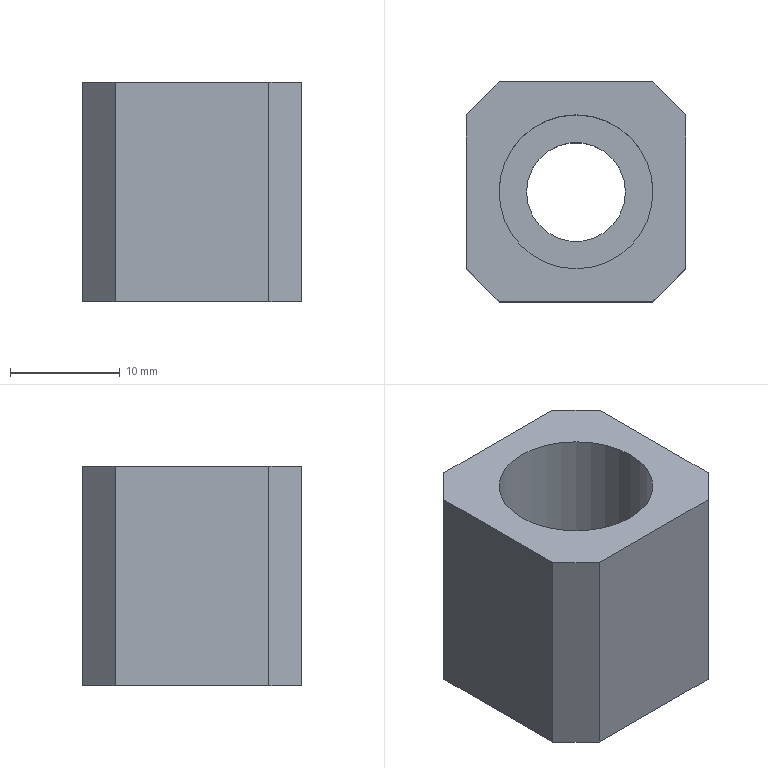Part | STEP file | 1_id270_x_t | 1 solid | 13 faces | box 20 x 20 x 20 mm | volume 5374 mm3 | plane 11 | cylinder 2 | commonest cylinder face diameters 9 x1 14 x1
STEP:
#1=CARTESIAN_POINT('',(0.,0.,0.));
#2=DIRECTION('',(0.,0.,1.));
#3=DIRECTION('',(1.,0.,0.));
#4=AXIS2_PLACEMENT_3D('',#1,#2,#3);
#5=CARTESIAN_POINT('',(740.075,184.5,-25.68));
#6=VERTEX_POINT('',#5);
#7=CARTESIAN_POINT('',(740.075,170.5,-25.68));
#8=VERTEX_POINT('',#7);
#9=CARTESIAN_POINT('',(740.075,188.5,-25.68));
#10=DIRECTION('',(0.,-1.,0.));
#11=VECTOR('',#10,1.);
#12=LINE('',#9,#11);
#13=CARTESIAN_POINT('',(740.075,188.5,-0.68));
#14=DIRECTION('',(1.,0.,0.));
#15=DIRECTION('',(0.,0.,-1.));
#16=AXIS2_PLACEMENT_3D('',#13,#14,#15);
#17=PLANE('',#16);
#18=CARTESIAN_POINT('',(25.,0.));
#19=DIRECTION('',(0.,-1.));
#20=VECTOR('',#19,1.);
#21=LINE('',#18,#20);
#22=(GEOMETRIC_REPRESENTATION_CONTEXT(2)PARAMETRIC_REPRESENTATION_CONTEXT()REPRESENTATION_CONTEXT('',''));
#23=DEFINITIONAL_REPRESENTATION('',(#21),#22);
#24=PCURVE('',#17,#23);
#25=CARTESIAN_POINT('',(740.075,166.5,-25.68));
#26=DIRECTION('',(0.,0.,1.));
#27=DIRECTION('',(1.,0.,0.));
#28=AXIS2_PLACEMENT_3D('',#25,#26,#27);
#29=PLANE('',#28);
#30=CARTESIAN_POINT('',(0.,22.));
#31=DIRECTION('',(0.,-1.));
#32=VECTOR('',#31,1.);
#33=LINE('',#30,#32);
#34=(GEOMETRIC_REPRESENTATION_CONTEXT(2)PARAMETRIC_REPRESENTATION_CONTEXT()REPRESENTATION_CONTEXT('',''));
#35=DEFINITIONAL_REPRESENTATION('',(#33),#34);
#36=PCURVE('',#29,#35);
#37=SURFACE_CURVE('',#12,(#24,#36),.PCURVE_S1.);
#38=EDGE_CURVE('',#6,#8,#37,.T.);
#39=ORIENTED_EDGE('',*,*,#38,.T.);
#40=CARTESIAN_POINT('',(740.075,170.5,-5.68));
#41=VERTEX_POINT('',#40);
#42=CARTESIAN_POINT('',(740.075,170.5,-0.68));
#43=DIRECTION('',(0.,0.,1.));
#44=VECTOR('',#43,1.);
#45=LINE('',#42,#44);
#46=CARTESIAN_POINT('',(0.,-18.));
#47=DIRECTION('',(-1.,0.));
#48=VECTOR('',#47,1.);
#49=LINE('',#46,#48);
#50=(GEOMETRIC_REPRESENTATION_CONTEXT(2)PARAMETRIC_REPRESENTATION_CONTEXT()REPRESENTATION_CONTEXT('',''));
#51=DEFINITIONAL_REPRESENTATION('',(#49),#50);
#52=PCURVE('',#17,#51);
#53=CARTESIAN_POINT('',(743.075,167.5,-0.68));
#54=DIRECTION('',(0.7071,0.7071,0.));
#55=DIRECTION('',(-0.7071,0.7071,0.));
#56=AXIS2_PLACEMENT_3D('',#53,#54,#55);
#57=PLANE('',#56);
#58=CARTESIAN_POINT('',(4.243,0.));
#59=DIRECTION('',(0.,1.));
#60=VECTOR('',#59,1.);
#61=LINE('',#58,#60);
#62=(GEOMETRIC_REPRESENTATION_CONTEXT(2)PARAMETRIC_REPRESENTATION_CONTEXT()REPRESENTATION_CONTEXT('',''));
#63=DEFINITIONAL_REPRESENTATION('',(#61),#62);
#64=PCURVE('',#57,#63);
#65=SURFACE_CURVE('',#45,(#52,#64),.PCURVE_S1.);
#66=EDGE_CURVE('',#8,#41,#65,.T.);
#67=ORIENTED_EDGE('',*,*,#66,.T.);
#68=CARTESIAN_POINT('',(740.075,184.5,-5.68));
#69=VERTEX_POINT('',#68);
#70=CARTESIAN_POINT('',(740.075,188.5,-5.68));
#71=DIRECTION('',(0.,-1.,0.));
#72=VECTOR('',#71,1.);
#73=LINE('',#70,#72);
#74=CARTESIAN_POINT('',(5.,0.));
#75=DIRECTION('',(0.,-1.));
#76=VECTOR('',#75,1.);
#77=LINE('',#74,#76);
#78=(GEOMETRIC_REPRESENTATION_CONTEXT(2)PARAMETRIC_REPRESENTATION_CONTEXT()REPRESENTATION_CONTEXT('',''));
#79=DEFINITIONAL_REPRESENTATION('',(#77),#78);
#80=PCURVE('',#17,#79);
#81=CARTESIAN_POINT('',(740.075,166.5,-5.68));
#82=DIRECTION('',(0.,0.,1.));
#83=DIRECTION('',(1.,0.,0.));
#84=AXIS2_PLACEMENT_3D('',#81,#82,#83);
#85=PLANE('',#84);
#86=CARTESIAN_POINT('',(0.,22.));
#87=DIRECTION('',(0.,-1.));
#88=VECTOR('',#87,1.);
#89=LINE('',#86,#88);
#90=(GEOMETRIC_REPRESENTATION_CONTEXT(2)PARAMETRIC_REPRESENTATION_CONTEXT()REPRESENTATION_CONTEXT('',''));
#91=DEFINITIONAL_REPRESENTATION('',(#89),#90);
#92=PCURVE('',#85,#91);
#93=SURFACE_CURVE('',#73,(#80,#92),.PCURVE_S1.);
#94=EDGE_CURVE('',#69,#41,#93,.T.);
#95=ORIENTED_EDGE('',*,*,#94,.F.);
#96=CARTESIAN_POINT('',(740.075,184.5,-0.68));
#97=DIRECTION('',(0.,0.,-1.));
#98=VECTOR('',#97,1.);
#99=LINE('',#96,#98);
#100=CARTESIAN_POINT('',(0.,-4.));
#101=DIRECTION('',(1.,0.));
#102=VECTOR('',#101,1.);
#103=LINE('',#100,#102);
#104=(GEOMETRIC_REPRESENTATION_CONTEXT(2)PARAMETRIC_REPRESENTATION_CONTEXT()REPRESENTATION_CONTEXT('',''));
#105=DEFINITIONAL_REPRESENTATION('',(#103),#104);
#106=PCURVE('',#17,#105);
#107=CARTESIAN_POINT('',(740.075,184.5,-0.68));
#108=DIRECTION('',(0.7071,-0.7071,0.));
#109=DIRECTION('',(0.7071,0.7071,0.));
#110=AXIS2_PLACEMENT_3D('',#107,#108,#109);
#111=PLANE('',#110);
#112=CARTESIAN_POINT('',(0.,0.));
#113=DIRECTION('',(0.,-1.));
#114=VECTOR('',#113,1.);
#115=LINE('',#112,#114);
#116=(GEOMETRIC_REPRESENTATION_CONTEXT(2)PARAMETRIC_REPRESENTATION_CONTEXT()REPRESENTATION_CONTEXT('',''));
#117=DEFINITIONAL_REPRESENTATION('',(#115),#116);
#118=PCURVE('',#111,#117);
#119=SURFACE_CURVE('',#99,(#106,#118),.PCURVE_S1.);
#120=EDGE_CURVE('',#69,#6,#119,.T.);
#121=ORIENTED_EDGE('',*,*,#120,.T.);
#122=EDGE_LOOP('',(#39,#67,#95,#121));
#123=FACE_BOUND('',#122,.T.);
#124=ADVANCED_FACE('',(#123),#17,.F.);
#125=CARTESIAN_POINT('',(743.075,167.5,-5.68));
#126=VERTEX_POINT('',#125);
#127=CARTESIAN_POINT('',(757.075,167.5,-5.68));
#128=VERTEX_POINT('',#127);
#129=CARTESIAN_POINT('',(740.075,167.5,-5.68));
#130=DIRECTION('',(1.,0.,0.));
#131=VECTOR('',#130,1.);
#132=LINE('',#129,#131);
#133=CARTESIAN_POINT('',(740.075,167.5,-0.68));
#134=DIRECTION('',(0.,1.,0.));
#135=DIRECTION('',(0.,0.,1.));
#136=AXIS2_PLACEMENT_3D('',#133,#134,#135);
#137=PLANE('',#136);
#138=CARTESIAN_POINT('',(-5.,0.));
#139=DIRECTION('',(0.,1.));
#140=VECTOR('',#139,1.);
#141=LINE('',#138,#140);
#142=(GEOMETRIC_REPRESENTATION_CONTEXT(2)PARAMETRIC_REPRESENTATION_CONTEXT()REPRESENTATION_CONTEXT('',''));
#143=DEFINITIONAL_REPRESENTATION('',(#141),#142);
#144=PCURVE('',#137,#143);
#145=CARTESIAN_POINT('',(0.,1.));
#146=DIRECTION('',(1.,0.));
#147=VECTOR('',#146,1.);
#148=LINE('',#145,#147);
#149=(GEOMETRIC_REPRESENTATION_CONTEXT(2)PARAMETRIC_REPRESENTATION_CONTEXT()REPRESENTATION_CONTEXT('',''));
#150=DEFINITIONAL_REPRESENTATION('',(#148),#149);
#151=PCURVE('',#85,#150);
#152=SURFACE_CURVE('',#132,(#144,#151),.PCURVE_S1.);
#153=EDGE_CURVE('',#126,#128,#152,.T.);
#154=ORIENTED_EDGE('',*,*,#153,.F.);
#155=CARTESIAN_POINT('',(743.075,167.5,-25.68));
#156=VERTEX_POINT('',#155);
#157=CARTESIAN_POINT('',(743.075,167.5,-0.68));
#158=DIRECTION('',(0.,0.,-1.));
#159=VECTOR('',#158,1.);
#160=LINE('',#157,#159);
#161=CARTESIAN_POINT('',(0.,3.));
#162=DIRECTION('',(-1.,0.));
#163=VECTOR('',#162,1.);
#164=LINE('',#161,#163);
#165=(GEOMETRIC_REPRESENTATION_CONTEXT(2)PARAMETRIC_REPRESENTATION_CONTEXT()REPRESENTATION_CONTEXT('',''));
#166=DEFINITIONAL_REPRESENTATION('',(#164),#165);
#167=PCURVE('',#137,#166);
#168=CARTESIAN_POINT('',(0.,0.));
#169=DIRECTION('',(0.,-1.));
#170=VECTOR('',#169,1.);
#171=LINE('',#168,#170);
#172=(GEOMETRIC_REPRESENTATION_CONTEXT(2)PARAMETRIC_REPRESENTATION_CONTEXT()REPRESENTATION_CONTEXT('',''));
#173=DEFINITIONAL_REPRESENTATION('',(#171),#172);
#174=PCURVE('',#57,#173);
#175=SURFACE_CURVE('',#160,(#167,#174),.PCURVE_S1.);
#176=EDGE_CURVE('',#126,#156,#175,.T.);
#177=ORIENTED_EDGE('',*,*,#176,.T.);
#178=CARTESIAN_POINT('',(757.075,167.5,-25.68));
#179=VERTEX_POINT('',#178);
#180=CARTESIAN_POINT('',(740.075,167.5,-25.68));
#181=DIRECTION('',(1.,0.,0.));
#182=VECTOR('',#181,1.);
#183=LINE('',#180,#182);
#184=CARTESIAN_POINT('',(-25.,0.));
#185=DIRECTION('',(0.,1.));
#186=VECTOR('',#185,1.);
#187=LINE('',#184,#186);
#188=(GEOMETRIC_REPRESENTATION_CONTEXT(2)PARAMETRIC_REPRESENTATION_CONTEXT()REPRESENTATION_CONTEXT('',''));
#189=DEFINITIONAL_REPRESENTATION('',(#187),#188);
#190=PCURVE('',#137,#189);
#191=CARTESIAN_POINT('',(0.,1.));
#192=DIRECTION('',(1.,0.));
#193=VECTOR('',#192,1.);
#194=LINE('',#191,#193);
#195=(GEOMETRIC_REPRESENTATION_CONTEXT(2)PARAMETRIC_REPRESENTATION_CONTEXT()REPRESENTATION_CONTEXT('',''));
#196=DEFINITIONAL_REPRESENTATION('',(#194),#195);
#197=PCURVE('',#29,#196);
#198=SURFACE_CURVE('',#183,(#190,#197),.PCURVE_S1.);
#199=EDGE_CURVE('',#156,#179,#198,.T.);
#200=ORIENTED_EDGE('',*,*,#199,.T.);
#201=CARTESIAN_POINT('',(757.075,167.5,-0.68));
#202=DIRECTION('',(0.,0.,1.));
#203=VECTOR('',#202,1.);
#204=LINE('',#201,#203);
#205=CARTESIAN_POINT('',(0.,17.));
#206=DIRECTION('',(1.,0.));
#207=VECTOR('',#206,1.);
#208=LINE('',#205,#207);
#209=(GEOMETRIC_REPRESENTATION_CONTEXT(2)PARAMETRIC_REPRESENTATION_CONTEXT()REPRESENTATION_CONTEXT('',''));
#210=DEFINITIONAL_REPRESENTATION('',(#208),#209);
#211=PCURVE('',#137,#210);
#212=CARTESIAN_POINT('',(760.075,170.5,-0.68));
#213=DIRECTION('',(-0.7071,0.7071,0.));
#214=DIRECTION('',(-0.7071,-0.7071,0.));
#215=AXIS2_PLACEMENT_3D('',#212,#213,#214);
#216=PLANE('',#215);
#217=CARTESIAN_POINT('',(4.243,0.));
#218=DIRECTION('',(0.,1.));
#219=VECTOR('',#218,1.);
#220=LINE('',#217,#219);
#221=(GEOMETRIC_REPRESENTATION_CONTEXT(2)PARAMETRIC_REPRESENTATION_CONTEXT()REPRESENTATION_CONTEXT('',''));
#222=DEFINITIONAL_REPRESENTATION('',(#220),#221);
#223=PCURVE('',#216,#222);
#224=SURFACE_CURVE('',#204,(#211,#223),.PCURVE_S1.);
#225=EDGE_CURVE('',#179,#128,#224,.T.);
#226=ORIENTED_EDGE('',*,*,#225,.T.);
#227=EDGE_LOOP('',(#154,#177,#200,#226));
#228=FACE_BOUND('',#227,.T.);
#229=ADVANCED_FACE('',(#228),#137,.F.);
#230=CARTESIAN_POINT('',(760.075,170.5,-5.68));
#231=VERTEX_POINT('',#230);
#232=CARTESIAN_POINT('',(760.075,184.5,-5.68));
#233=VERTEX_POINT('',#232);
#234=CARTESIAN_POINT('',(760.075,166.5,-5.68));
#235=DIRECTION('',(0.,1.,0.));
#236=VECTOR('',#235,1.);
#237=LINE('',#234,#236);
#238=CARTESIAN_POINT('',(760.075,166.5,-0.68));
#239=DIRECTION('',(-1.,0.,0.));
#240=DIRECTION('',(0.,0.,1.));
#241=AXIS2_PLACEMENT_3D('',#238,#239,#240);
#242=PLANE('',#241);
#243=CARTESIAN_POINT('',(-5.,0.));
#244=DIRECTION('',(0.,1.));
#245=VECTOR('',#244,1.);
#246=LINE('',#243,#245);
#247=(GEOMETRIC_REPRESENTATION_CONTEXT(2)PARAMETRIC_REPRESENTATION_CONTEXT()REPRESENTATION_CONTEXT('',''));
#248=DEFINITIONAL_REPRESENTATION('',(#246),#247);
#249=PCURVE('',#242,#248);
#250=CARTESIAN_POINT('',(20.,0.));
#251=DIRECTION('',(0.,1.));
#252=VECTOR('',#251,1.);
#253=LINE('',#250,#252);
#254=(GEOMETRIC_REPRESENTATION_CONTEXT(2)PARAMETRIC_REPRESENTATION_CONTEXT()REPRESENTATION_CONTEXT('',''));
#255=DEFINITIONAL_REPRESENTATION('',(#253),#254);
#256=PCURVE('',#85,#255);
#257=SURFACE_CURVE('',#237,(#249,#256),.PCURVE_S1.);
#258=EDGE_CURVE('',#231,#233,#257,.T.);
#259=ORIENTED_EDGE('',*,*,#258,.F.);
#260=CARTESIAN_POINT('',(760.075,170.5,-25.68));
#261=VERTEX_POINT('',#260);
#262=CARTESIAN_POINT('',(760.075,170.5,-0.68));
#263=DIRECTION('',(0.,0.,-1.));
#264=VECTOR('',#263,1.);
#265=LINE('',#262,#264);
#266=CARTESIAN_POINT('',(0.,4.));
#267=DIRECTION('',(-1.,0.));
#268=VECTOR('',#267,1.);
#269=LINE('',#266,#268);
#270=(GEOMETRIC_REPRESENTATION_CONTEXT(2)PARAMETRIC_REPRESENTATION_CONTEXT()REPRESENTATION_CONTEXT('',''));
#271=DEFINITIONAL_REPRESENTATION('',(#269),#270);
#272=PCURVE('',#242,#271);
#273=CARTESIAN_POINT('',(0.,0.));
#274=DIRECTION('',(0.,-1.));
#275=VECTOR('',#274,1.);
#276=LINE('',#273,#275);
#277=(GEOMETRIC_REPRESENTATION_CONTEXT(2)PARAMETRIC_REPRESENTATION_CONTEXT()REPRESENTATION_CONTEXT('',''));
#278=DEFINITIONAL_REPRESENTATION('',(#276),#277);
#279=PCURVE('',#216,#278);
#280=SURFACE_CURVE('',#265,(#272,#279),.PCURVE_S1.);
#281=EDGE_CURVE('',#231,#261,#280,.T.);
#282=ORIENTED_EDGE('',*,*,#281,.T.);
#283=CARTESIAN_POINT('',(760.075,184.5,-25.68));
#284=VERTEX_POINT('',#283);
#285=CARTESIAN_POINT('',(760.075,166.5,-25.68));
#286=DIRECTION('',(0.,1.,0.));
#287=VECTOR('',#286,1.);
#288=LINE('',#285,#287);
#289=CARTESIAN_POINT('',(-25.,0.));
#290=DIRECTION('',(0.,1.));
#291=VECTOR('',#290,1.);
#292=LINE('',#289,#291);
#293=(GEOMETRIC_REPRESENTATION_CONTEXT(2)PARAMETRIC_REPRESENTATION_CONTEXT()REPRESENTATION_CONTEXT('',''));
#294=DEFINITIONAL_REPRESENTATION('',(#292),#293);
#295=PCURVE('',#242,#294);
#296=CARTESIAN_POINT('',(20.,0.));
#297=DIRECTION('',(0.,1.));
#298=VECTOR('',#297,1.);
#299=LINE('',#296,#298);
#300=(GEOMETRIC_REPRESENTATION_CONTEXT(2)PARAMETRIC_REPRESENTATION_CONTEXT()REPRESENTATION_CONTEXT('',''));
#301=DEFINITIONAL_REPRESENTATION('',(#299),#300);
#302=PCURVE('',#29,#301);
#303=SURFACE_CURVE('',#288,(#295,#302),.PCURVE_S1.);
#304=EDGE_CURVE('',#261,#284,#303,.T.);
#305=ORIENTED_EDGE('',*,*,#304,.T.);
#306=CARTESIAN_POINT('',(760.075,184.5,-0.68));
#307=DIRECTION('',(0.,0.,1.));
#308=VECTOR('',#307,1.);
#309=LINE('',#306,#308);
#310=CARTESIAN_POINT('',(0.,18.));
#311=DIRECTION('',(1.,0.));
#312=VECTOR('',#311,1.);
#313=LINE('',#310,#312);
#314=(GEOMETRIC_REPRESENTATION_CONTEXT(2)PARAMETRIC_REPRESENTATION_CONTEXT()REPRESENTATION_CONTEXT('',''));
#315=DEFINITIONAL_REPRESENTATION('',(#313),#314);
#316=PCURVE('',#242,#315);
#317=CARTESIAN_POINT('',(757.075,187.5,-0.68));
#318=DIRECTION('',(-0.7071,-0.7071,0.));
#319=DIRECTION('',(0.7071,-0.7071,0.));
#320=AXIS2_PLACEMENT_3D('',#317,#318,#319);
#321=PLANE('',#320);
#322=CARTESIAN_POINT('',(4.243,0.));
#323=DIRECTION('',(0.,1.));
#324=VECTOR('',#323,1.);
#325=LINE('',#322,#324);
#326=(GEOMETRIC_REPRESENTATION_CONTEXT(2)PARAMETRIC_REPRESENTATION_CONTEXT()REPRESENTATION_CONTEXT('',''));
#327=DEFINITIONAL_REPRESENTATION('',(#325),#326);
#328=PCURVE('',#321,#327);
#329=SURFACE_CURVE('',#309,(#316,#328),.PCURVE_S1.);
#330=EDGE_CURVE('',#284,#233,#329,.T.);
#331=ORIENTED_EDGE('',*,*,#330,.T.);
#332=EDGE_LOOP('',(#259,#282,#305,#331));
#333=FACE_BOUND('',#332,.T.);
#334=ADVANCED_FACE('',(#333),#242,.F.);
#335=CARTESIAN_POINT('',(757.075,187.5,-25.68));
#336=VERTEX_POINT('',#335);
#337=CARTESIAN_POINT('',(743.075,187.5,-25.68));
#338=VERTEX_POINT('',#337);
#339=CARTESIAN_POINT('',(760.075,187.5,-25.68));
#340=DIRECTION('',(-1.,0.,0.));
#341=VECTOR('',#340,1.);
#342=LINE('',#339,#341);
#343=CARTESIAN_POINT('',(760.075,187.5,-0.68));
#344=DIRECTION('',(0.,-1.,0.));
#345=DIRECTION('',(0.,0.,-1.));
#346=AXIS2_PLACEMENT_3D('',#343,#344,#345);
#347=PLANE('',#346);
#348=CARTESIAN_POINT('',(25.,0.));
#349=DIRECTION('',(0.,-1.));
#350=VECTOR('',#349,1.);
#351=LINE('',#348,#350);
#352=(GEOMETRIC_REPRESENTATION_CONTEXT(2)PARAMETRIC_REPRESENTATION_CONTEXT()REPRESENTATION_CONTEXT('',''));
#353=DEFINITIONAL_REPRESENTATION('',(#351),#352);
#354=PCURVE('',#347,#353);
#355=CARTESIAN_POINT('',(20.,21.));
#356=DIRECTION('',(-1.,0.));
#357=VECTOR('',#356,1.);
#358=LINE('',#355,#357);
#359=(GEOMETRIC_REPRESENTATION_CONTEXT(2)PARAMETRIC_REPRESENTATION_CONTEXT()REPRESENTATION_CONTEXT('',''));
#360=DEFINITIONAL_REPRESENTATION('',(#358),#359);
#361=PCURVE('',#29,#360);
#362=SURFACE_CURVE('',#342,(#354,#361),.PCURVE_S1.);
#363=EDGE_CURVE('',#336,#338,#362,.T.);
#364=ORIENTED_EDGE('',*,*,#363,.T.);
#365=CARTESIAN_POINT('',(743.075,187.5,-5.68));
#366=VERTEX_POINT('',#365);
#367=CARTESIAN_POINT('',(743.075,187.5,-0.68));
#368=DIRECTION('',(0.,0.,1.));
#369=VECTOR('',#368,1.);
#370=LINE('',#367,#369);
#371=CARTESIAN_POINT('',(0.,-17.));
#372=DIRECTION('',(-1.,0.));
#373=VECTOR('',#372,1.);
#374=LINE('',#371,#373);
#375=(GEOMETRIC_REPRESENTATION_CONTEXT(2)PARAMETRIC_REPRESENTATION_CONTEXT()REPRESENTATION_CONTEXT('',''));
#376=DEFINITIONAL_REPRESENTATION('',(#374),#375);
#377=PCURVE('',#347,#376);
#378=CARTESIAN_POINT('',(4.243,0.));
#379=DIRECTION('',(0.,1.));
#380=VECTOR('',#379,1.);
#381=LINE('',#378,#380);
#382=(GEOMETRIC_REPRESENTATION_CONTEXT(2)PARAMETRIC_REPRESENTATION_CONTEXT()REPRESENTATION_CONTEXT('',''));
#383=DEFINITIONAL_REPRESENTATION('',(#381),#382);
#384=PCURVE('',#111,#383);
#385=SURFACE_CURVE('',#370,(#377,#384),.PCURVE_S1.);
#386=EDGE_CURVE('',#338,#366,#385,.T.);
#387=ORIENTED_EDGE('',*,*,#386,.T.);
#388=CARTESIAN_POINT('',(757.075,187.5,-5.68));
#389=VERTEX_POINT('',#388);
#390=CARTESIAN_POINT('',(760.075,187.5,-5.68));
#391=DIRECTION('',(-1.,0.,0.));
#392=VECTOR('',#391,1.);
#393=LINE('',#390,#392);
#394=CARTESIAN_POINT('',(5.,0.));
#395=DIRECTION('',(0.,-1.));
#396=VECTOR('',#395,1.);
#397=LINE('',#394,#396);
#398=(GEOMETRIC_REPRESENTATION_CONTEXT(2)PARAMETRIC_REPRESENTATION_CONTEXT()REPRESENTATION_CONTEXT('',''));
#399=DEFINITIONAL_REPRESENTATION('',(#397),#398);
#400=PCURVE('',#347,#399);
#401=CARTESIAN_POINT('',(20.,21.));
#402=DIRECTION('',(-1.,0.));
#403=VECTOR('',#402,1.);
#404=LINE('',#401,#403);
#405=(GEOMETRIC_REPRESENTATION_CONTEXT(2)PARAMETRIC_REPRESENTATION_CONTEXT()REPRESENTATION_CONTEXT('',''));
#406=DEFINITIONAL_REPRESENTATION('',(#404),#405);
#407=PCURVE('',#85,#406);
#408=SURFACE_CURVE('',#393,(#400,#407),.PCURVE_S1.);
#409=EDGE_CURVE('',#389,#366,#408,.T.);
#410=ORIENTED_EDGE('',*,*,#409,.F.);
#411=CARTESIAN_POINT('',(757.075,187.5,-0.68));
#412=DIRECTION('',(0.,0.,-1.));
#413=VECTOR('',#412,1.);
#414=LINE('',#411,#413);
#415=CARTESIAN_POINT('',(0.,-3.));
#416=DIRECTION('',(1.,0.));
#417=VECTOR('',#416,1.);
#418=LINE('',#415,#417);
#419=(GEOMETRIC_REPRESENTATION_CONTEXT(2)PARAMETRIC_REPRESENTATION_CONTEXT()REPRESENTATION_CONTEXT('',''));
#420=DEFINITIONAL_REPRESENTATION('',(#418),#419);
#421=PCURVE('',#347,#420);
#422=CARTESIAN_POINT('',(0.,0.));
#423=DIRECTION('',(0.,-1.));
#424=VECTOR('',#423,1.);
#425=LINE('',#422,#424);
#426=(GEOMETRIC_REPRESENTATION_CONTEXT(2)PARAMETRIC_REPRESENTATION_CONTEXT()REPRESENTATION_CONTEXT('',''));
#427=DEFINITIONAL_REPRESENTATION('',(#425),#426);
#428=PCURVE('',#321,#427);
#429=SURFACE_CURVE('',#414,(#421,#428),.PCURVE_S1.);
#430=EDGE_CURVE('',#389,#336,#429,.T.);
#431=ORIENTED_EDGE('',*,*,#430,.T.);
#432=EDGE_LOOP('',(#364,#387,#410,#431));
#433=FACE_BOUND('',#432,.T.);
#434=ADVANCED_FACE('',(#433),#347,.F.);
#435=CARTESIAN_POINT('',(743.075,177.5,-5.68));
#436=VERTEX_POINT('',#435);
#437=CARTESIAN_POINT('',(750.075,177.5,-5.68));
#438=DIRECTION('',(0.,0.,-1.));
#439=DIRECTION('',(-1.,0.,0.));
#440=AXIS2_PLACEMENT_3D('',#437,#438,#439);
#441=CIRCLE('',#440,7.);
#442=CARTESIAN_POINT('',(3.,11.));
#443=CARTESIAN_POINT('',(3.,23.124));
#444=CARTESIAN_POINT('',(13.5,17.062));
#445=CARTESIAN_POINT('',(24.,11.));
#446=CARTESIAN_POINT('',(13.5,4.938));
#447=CARTESIAN_POINT('',(3.,-1.124));
#448=CARTESIAN_POINT('',(3.,11.));
#449=(BOUNDED_CURVE()B_SPLINE_CURVE(2,(#442,#443,#444,#445,#446,#447,#448),.UNSPECIFIED.,.T.,.F.)B_SPLINE_CURVE_WITH_KNOTS((1,2,2,2,2,1),(-2.094,0.,2.094,4.189,6.283,8.378),.UNSPECIFIED.)CURVE()GEOMETRIC_REPRESENTATION_ITEM()RATIONAL_B_SPLINE_CURVE((1.,0.5,1.,0.5,1.,0.5,1.))REPRESENTATION_ITEM(''));
#450=(GEOMETRIC_REPRESENTATION_CONTEXT(2)PARAMETRIC_REPRESENTATION_CONTEXT()REPRESENTATION_CONTEXT('',''));
#451=DEFINITIONAL_REPRESENTATION('',(#449),#450);
#452=PCURVE('',#85,#451);
#453=CARTESIAN_POINT('',(750.075,177.5,-5.68));
#454=DIRECTION('',(0.,0.,-1.));
#455=DIRECTION('',(-1.,0.,0.));
#456=AXIS2_PLACEMENT_3D('',#453,#454,#455);
#457=CYLINDRICAL_SURFACE('',#456,7.);
#458=CARTESIAN_POINT('',(0.,0.));
#459=DIRECTION('',(1.,0.));
#460=VECTOR('',#459,1.);
#461=LINE('',#458,#460);
#462=(GEOMETRIC_REPRESENTATION_CONTEXT(2)PARAMETRIC_REPRESENTATION_CONTEXT()REPRESENTATION_CONTEXT('',''));
#463=DEFINITIONAL_REPRESENTATION('',(#461),#462);
#464=PCURVE('',#457,#463);
#465=SURFACE_CURVE('',#441,(#452,#464),.PCURVE_S1.);
#466=EDGE_CURVE('',#436,#436,#465,.T.);
#467=ORIENTED_EDGE('',*,*,#466,.T.);
#468=EDGE_LOOP('',(#467));
#469=FACE_BOUND('',#468,.T.);
#470=ORIENTED_EDGE('',*,*,#94,.T.);
#471=CARTESIAN_POINT('',(742.075,168.5,-5.68));
#472=DIRECTION('',(0.7071,-0.7071,0.));
#473=VECTOR('',#472,1.);
#474=LINE('',#471,#473);
#475=CARTESIAN_POINT('',(2.,2.));
#476=DIRECTION('',(0.7071,-0.7071));
#477=VECTOR('',#476,1.);
#478=LINE('',#475,#477);
#479=(GEOMETRIC_REPRESENTATION_CONTEXT(2)PARAMETRIC_REPRESENTATION_CONTEXT()REPRESENTATION_CONTEXT('',''));
#480=DEFINITIONAL_REPRESENTATION('',(#478),#479);
#481=PCURVE('',#85,#480);
#482=CARTESIAN_POINT('',(1.414,-5.));
#483=DIRECTION('',(-1.,0.));
#484=VECTOR('',#483,1.);
#485=LINE('',#482,#484);
#486=(GEOMETRIC_REPRESENTATION_CONTEXT(2)PARAMETRIC_REPRESENTATION_CONTEXT()REPRESENTATION_CONTEXT('',''));
#487=DEFINITIONAL_REPRESENTATION('',(#485),#486);
#488=PCURVE('',#57,#487);
#489=SURFACE_CURVE('',#474,(#481,#488),.PCURVE_S1.);
#490=EDGE_CURVE('',#41,#126,#489,.T.);
#491=ORIENTED_EDGE('',*,*,#490,.T.);
#492=ORIENTED_EDGE('',*,*,#153,.T.);
#493=CARTESIAN_POINT('',(748.075,158.5,-5.68));
#494=DIRECTION('',(0.7071,0.7071,0.));
#495=VECTOR('',#494,1.);
#496=LINE('',#493,#495);
#497=CARTESIAN_POINT('',(8.,-8.));
#498=DIRECTION('',(0.7071,0.7071));
#499=VECTOR('',#498,1.);
#500=LINE('',#497,#499);
#501=(GEOMETRIC_REPRESENTATION_CONTEXT(2)PARAMETRIC_REPRESENTATION_CONTEXT()REPRESENTATION_CONTEXT('',''));
#502=DEFINITIONAL_REPRESENTATION('',(#500),#501);
#503=PCURVE('',#85,#502);
#504=CARTESIAN_POINT('',(16.971,-5.));
#505=DIRECTION('',(-1.,0.));
#506=VECTOR('',#505,1.);
#507=LINE('',#504,#506);
#508=(GEOMETRIC_REPRESENTATION_CONTEXT(2)PARAMETRIC_REPRESENTATION_CONTEXT()REPRESENTATION_CONTEXT('',''));
#509=DEFINITIONAL_REPRESENTATION('',(#507),#508);
#510=PCURVE('',#216,#509);
#511=SURFACE_CURVE('',#496,(#503,#510),.PCURVE_S1.);
#512=EDGE_CURVE('',#128,#231,#511,.T.);
#513=ORIENTED_EDGE('',*,*,#512,.T.);
#514=ORIENTED_EDGE('',*,*,#258,.T.);
#515=CARTESIAN_POINT('',(759.075,185.5,-5.68));
#516=DIRECTION('',(-0.7071,0.7071,0.));
#517=VECTOR('',#516,1.);
#518=LINE('',#515,#517);
#519=CARTESIAN_POINT('',(19.,19.));
#520=DIRECTION('',(-0.7071,0.7071));
#521=VECTOR('',#520,1.);
#522=LINE('',#519,#521);
#523=(GEOMETRIC_REPRESENTATION_CONTEXT(2)PARAMETRIC_REPRESENTATION_CONTEXT()REPRESENTATION_CONTEXT('',''));
#524=DEFINITIONAL_REPRESENTATION('',(#522),#523);
#525=PCURVE('',#85,#524);
#526=CARTESIAN_POINT('',(2.828,-5.));
#527=DIRECTION('',(-1.,0.));
#528=VECTOR('',#527,1.);
#529=LINE('',#526,#528);
#530=(GEOMETRIC_REPRESENTATION_CONTEXT(2)PARAMETRIC_REPRESENTATION_CONTEXT()REPRESENTATION_CONTEXT('',''));
#531=DEFINITIONAL_REPRESENTATION('',(#529),#530);
#532=PCURVE('',#321,#531);
#533=SURFACE_CURVE('',#518,(#525,#532),.PCURVE_S1.);
#534=EDGE_CURVE('',#233,#389,#533,.T.);
#535=ORIENTED_EDGE('',*,*,#534,.T.);
#536=ORIENTED_EDGE('',*,*,#409,.T.);
#537=CARTESIAN_POINT('',(731.075,175.5,-5.68));
#538=DIRECTION('',(-0.7071,-0.7071,0.));
#539=VECTOR('',#538,1.);
#540=LINE('',#537,#539);
#541=CARTESIAN_POINT('',(-9.,9.));
#542=DIRECTION('',(-0.7071,-0.7071));
#543=VECTOR('',#542,1.);
#544=LINE('',#541,#543);
#545=(GEOMETRIC_REPRESENTATION_CONTEXT(2)PARAMETRIC_REPRESENTATION_CONTEXT()REPRESENTATION_CONTEXT('',''));
#546=DEFINITIONAL_REPRESENTATION('',(#544),#545);
#547=PCURVE('',#85,#546);
#548=CARTESIAN_POINT('',(-12.728,-5.));
#549=DIRECTION('',(-1.,0.));
#550=VECTOR('',#549,1.);
#551=LINE('',#548,#550);
#552=(GEOMETRIC_REPRESENTATION_CONTEXT(2)PARAMETRIC_REPRESENTATION_CONTEXT()REPRESENTATION_CONTEXT('',''));
#553=DEFINITIONAL_REPRESENTATION('',(#551),#552);
#554=PCURVE('',#111,#553);
#555=SURFACE_CURVE('',#540,(#547,#554),.PCURVE_S1.);
#556=EDGE_CURVE('',#366,#69,#555,.T.);
#557=ORIENTED_EDGE('',*,*,#556,.T.);
#558=EDGE_LOOP('',(#470,#491,#492,#513,#514,#535,#536,#557));
#559=FACE_BOUND('',#558,.T.);
#560=ADVANCED_FACE('',(#469,#559),#85,.T.);
#561=CARTESIAN_POINT('',(754.575,177.5,-25.68));
#562=VERTEX_POINT('',#561);
#563=CARTESIAN_POINT('',(745.575,177.5,-25.68));
#564=VERTEX_POINT('',#563);
#565=CARTESIAN_POINT('',(750.075,177.5,-25.68));
#566=DIRECTION('',(0.,0.,1.));
#567=DIRECTION('',(1.,0.,0.));
#568=AXIS2_PLACEMENT_3D('',#565,#566,#567);
#569=CIRCLE('',#568,4.5);
#570=CARTESIAN_POINT('',(10.,11.));
#571=DIRECTION('',(1.,0.));
#572=AXIS2_PLACEMENT_2D('',#570,#571);
#573=CIRCLE('',#572,4.5);
#574=(GEOMETRIC_REPRESENTATION_CONTEXT(2)PARAMETRIC_REPRESENTATION_CONTEXT()REPRESENTATION_CONTEXT('',''));
#575=DEFINITIONAL_REPRESENTATION('',(#573),#574);
#576=PCURVE('',#29,#575);
#577=CARTESIAN_POINT('',(750.075,177.5,-105.68));
#578=DIRECTION('',(0.,0.,-1.));
#579=DIRECTION('',(-1.,0.,0.));
#580=AXIS2_PLACEMENT_3D('',#577,#578,#579);
#581=CYLINDRICAL_SURFACE('',#580,4.5);
#582=CARTESIAN_POINT('',(3.142,-80.));
#583=DIRECTION('',(-1.,0.));
#584=VECTOR('',#583,1.);
#585=LINE('',#582,#584);
#586=(GEOMETRIC_REPRESENTATION_CONTEXT(2)PARAMETRIC_REPRESENTATION_CONTEXT()REPRESENTATION_CONTEXT('',''));
#587=DEFINITIONAL_REPRESENTATION('',(#585),#586);
#588=PCURVE('',#581,#587);
#589=SURFACE_CURVE('',#569,(#576,#588),.PCURVE_S1.);
#590=EDGE_CURVE('',#562,#564,#589,.T.);
#591=ORIENTED_EDGE('',*,*,#590,.T.);
#592=CARTESIAN_POINT('',(750.075,177.5,-25.68));
#593=DIRECTION('',(0.,0.,1.));
#594=DIRECTION('',(1.,0.,0.));
#595=AXIS2_PLACEMENT_3D('',#592,#593,#594);
#596=CIRCLE('',#595,4.5);
#597=CARTESIAN_POINT('',(10.,11.));
#598=DIRECTION('',(1.,0.));
#599=AXIS2_PLACEMENT_2D('',#597,#598);
#600=CIRCLE('',#599,4.5);
#601=(GEOMETRIC_REPRESENTATION_CONTEXT(2)PARAMETRIC_REPRESENTATION_CONTEXT()REPRESENTATION_CONTEXT('',''));
#602=DEFINITIONAL_REPRESENTATION('',(#600),#601);
#603=PCURVE('',#29,#602);
#604=CARTESIAN_POINT('',(9.425,-80.));
#605=DIRECTION('',(-1.,0.));
#606=VECTOR('',#605,1.);
#607=LINE('',#604,#606);
#608=(GEOMETRIC_REPRESENTATION_CONTEXT(2)PARAMETRIC_REPRESENTATION_CONTEXT()REPRESENTATION_CONTEXT('',''));
#609=DEFINITIONAL_REPRESENTATION('',(#607),#608);
#610=PCURVE('',#581,#609);
#611=SURFACE_CURVE('',#596,(#603,#610),.PCURVE_S1.);
#612=EDGE_CURVE('',#564,#562,#611,.T.);
#613=ORIENTED_EDGE('',*,*,#612,.T.);
#614=EDGE_LOOP('',(#591,#613));
#615=FACE_BOUND('',#614,.T.);
#616=ORIENTED_EDGE('',*,*,#199,.F.);
#617=CARTESIAN_POINT('',(743.075,167.5,-25.68));
#618=DIRECTION('',(-0.7071,0.7071,0.));
#619=VECTOR('',#618,1.);
#620=LINE('',#617,#619);
#621=CARTESIAN_POINT('',(3.,1.));
#622=DIRECTION('',(-0.7071,0.7071));
#623=VECTOR('',#622,1.);
#624=LINE('',#621,#623);
#625=(GEOMETRIC_REPRESENTATION_CONTEXT(2)PARAMETRIC_REPRESENTATION_CONTEXT()REPRESENTATION_CONTEXT('',''));
#626=DEFINITIONAL_REPRESENTATION('',(#624),#625);
#627=PCURVE('',#29,#626);
#628=CARTESIAN_POINT('',(0.,-25.));
#629=DIRECTION('',(1.,0.));
#630=VECTOR('',#629,1.);
#631=LINE('',#628,#630);
#632=(GEOMETRIC_REPRESENTATION_CONTEXT(2)PARAMETRIC_REPRESENTATION_CONTEXT()REPRESENTATION_CONTEXT('',''));
#633=DEFINITIONAL_REPRESENTATION('',(#631),#632);
#634=PCURVE('',#57,#633);
#635=SURFACE_CURVE('',#620,(#627,#634),.PCURVE_S1.);
#636=EDGE_CURVE('',#156,#8,#635,.T.);
#637=ORIENTED_EDGE('',*,*,#636,.T.);
#638=ORIENTED_EDGE('',*,*,#38,.F.);
#639=CARTESIAN_POINT('',(740.075,184.5,-25.68));
#640=DIRECTION('',(0.7071,0.7071,0.));
#641=VECTOR('',#640,1.);
#642=LINE('',#639,#641);
#643=CARTESIAN_POINT('',(0.,18.));
#644=DIRECTION('',(0.7071,0.7071));
#645=VECTOR('',#644,1.);
#646=LINE('',#643,#645);
#647=(GEOMETRIC_REPRESENTATION_CONTEXT(2)PARAMETRIC_REPRESENTATION_CONTEXT()REPRESENTATION_CONTEXT('',''));
#648=DEFINITIONAL_REPRESENTATION('',(#646),#647);
#649=PCURVE('',#29,#648);
#650=CARTESIAN_POINT('',(0.,-25.));
#651=DIRECTION('',(1.,0.));
#652=VECTOR('',#651,1.);
#653=LINE('',#650,#652);
#654=(GEOMETRIC_REPRESENTATION_CONTEXT(2)PARAMETRIC_REPRESENTATION_CONTEXT()REPRESENTATION_CONTEXT('',''));
#655=DEFINITIONAL_REPRESENTATION('',(#653),#654);
#656=PCURVE('',#111,#655);
#657=SURFACE_CURVE('',#642,(#649,#656),.PCURVE_S1.);
#658=EDGE_CURVE('',#6,#338,#657,.T.);
#659=ORIENTED_EDGE('',*,*,#658,.T.);
#660=ORIENTED_EDGE('',*,*,#363,.F.);
#661=CARTESIAN_POINT('',(757.075,187.5,-25.68));
#662=DIRECTION('',(0.7071,-0.7071,0.));
#663=VECTOR('',#662,1.);
#664=LINE('',#661,#663);
#665=CARTESIAN_POINT('',(17.,21.));
#666=DIRECTION('',(0.7071,-0.7071));
#667=VECTOR('',#666,1.);
#668=LINE('',#665,#667);
#669=(GEOMETRIC_REPRESENTATION_CONTEXT(2)PARAMETRIC_REPRESENTATION_CONTEXT()REPRESENTATION_CONTEXT('',''));
#670=DEFINITIONAL_REPRESENTATION('',(#668),#669);
#671=PCURVE('',#29,#670);
#672=CARTESIAN_POINT('',(0.,-25.));
#673=DIRECTION('',(1.,0.));
#674=VECTOR('',#673,1.);
#675=LINE('',#672,#674);
#676=(GEOMETRIC_REPRESENTATION_CONTEXT(2)PARAMETRIC_REPRESENTATION_CONTEXT()REPRESENTATION_CONTEXT('',''));
#677=DEFINITIONAL_REPRESENTATION('',(#675),#676);
#678=PCURVE('',#321,#677);
#679=SURFACE_CURVE('',#664,(#671,#678),.PCURVE_S1.);
#680=EDGE_CURVE('',#336,#284,#679,.T.);
#681=ORIENTED_EDGE('',*,*,#680,.T.);
#682=ORIENTED_EDGE('',*,*,#304,.F.);
#683=CARTESIAN_POINT('',(760.075,170.5,-25.68));
#684=DIRECTION('',(-0.7071,-0.7071,0.));
#685=VECTOR('',#684,1.);
#686=LINE('',#683,#685);
#687=CARTESIAN_POINT('',(20.,4.));
#688=DIRECTION('',(-0.7071,-0.7071));
#689=VECTOR('',#688,1.);
#690=LINE('',#687,#689);
#691=(GEOMETRIC_REPRESENTATION_CONTEXT(2)PARAMETRIC_REPRESENTATION_CONTEXT()REPRESENTATION_CONTEXT('',''));
#692=DEFINITIONAL_REPRESENTATION('',(#690),#691);
#693=PCURVE('',#29,#692);
#694=CARTESIAN_POINT('',(0.,-25.));
#695=DIRECTION('',(1.,0.));
#696=VECTOR('',#695,1.);
#697=LINE('',#694,#696);
#698=(GEOMETRIC_REPRESENTATION_CONTEXT(2)PARAMETRIC_REPRESENTATION_CONTEXT()REPRESENTATION_CONTEXT('',''));
#699=DEFINITIONAL_REPRESENTATION('',(#697),#698);
#700=PCURVE('',#216,#699);
#701=SURFACE_CURVE('',#686,(#693,#700),.PCURVE_S1.);
#702=EDGE_CURVE('',#261,#179,#701,.T.);
#703=ORIENTED_EDGE('',*,*,#702,.T.);
#704=EDGE_LOOP('',(#616,#637,#638,#659,#660,#681,#682,#703));
#705=FACE_BOUND('',#704,.T.);
#706=ADVANCED_FACE('',(#615,#705),#29,.F.);
#707=CARTESIAN_POINT('',(745.575,177.5,-16.68));
#708=VERTEX_POINT('',#707);
#709=CARTESIAN_POINT('',(750.075,177.5,-16.68));
#710=DIRECTION('',(0.,0.,-1.));
#711=DIRECTION('',(-1.,0.,0.));
#712=AXIS2_PLACEMENT_3D('',#709,#710,#711);
#713=CIRCLE('',#712,4.5);
#714=CARTESIAN_POINT('',(0.,-89.));
#715=DIRECTION('',(1.,0.));
#716=VECTOR('',#715,1.);
#717=LINE('',#714,#716);
#718=(GEOMETRIC_REPRESENTATION_CONTEXT(2)PARAMETRIC_REPRESENTATION_CONTEXT()REPRESENTATION_CONTEXT('',''));
#719=DEFINITIONAL_REPRESENTATION('',(#717),#718);
#720=PCURVE('',#581,#719);
#721=CARTESIAN_POINT('',(750.075,177.5,-16.68));
#722=DIRECTION('',(0.,0.,-1.));
#723=DIRECTION('',(-1.,0.,0.));
#724=AXIS2_PLACEMENT_3D('',#721,#722,#723);
#725=PLANE('',#724);
#726=CARTESIAN_POINT('',(0.,0.));
#727=DIRECTION('',(1.,0.));
#728=AXIS2_PLACEMENT_2D('',#726,#727);
#729=CIRCLE('',#728,4.5);
#730=(GEOMETRIC_REPRESENTATION_CONTEXT(2)PARAMETRIC_REPRESENTATION_CONTEXT()REPRESENTATION_CONTEXT('',''));
#731=DEFINITIONAL_REPRESENTATION('',(#729),#730);
#732=PCURVE('',#725,#731);
#733=SURFACE_CURVE('',#713,(#720,#732),.PCURVE_S1.);
#734=EDGE_CURVE('',#708,#708,#733,.T.);
#735=ORIENTED_EDGE('',*,*,#734,.T.);
#736=CARTESIAN_POINT('',(745.575,177.5,-16.68));
#737=CARTESIAN_POINT('',(745.575,177.5,-25.68));
#738=B_SPLINE_CURVE_WITH_KNOTS('',1,(#736,#737),.UNSPECIFIED.,.F.,.F.,(2,2),(-89.,-80.),.PIECEWISE_BEZIER_KNOTS.);
#739=CARTESIAN_POINT('',(6.283,0.));
#740=DIRECTION('',(0.,1.));
#741=VECTOR('',#740,1.);
#742=LINE('',#739,#741);
#743=(GEOMETRIC_REPRESENTATION_CONTEXT(2)PARAMETRIC_REPRESENTATION_CONTEXT()REPRESENTATION_CONTEXT('',''));
#744=DEFINITIONAL_REPRESENTATION('',(#742),#743);
#745=PCURVE('',#581,#744);
#746=CARTESIAN_POINT('',(0.,0.));
#747=DIRECTION('',(0.,1.));
#748=VECTOR('',#747,1.);
#749=LINE('',#746,#748);
#750=(GEOMETRIC_REPRESENTATION_CONTEXT(2)PARAMETRIC_REPRESENTATION_CONTEXT()REPRESENTATION_CONTEXT('',''));
#751=DEFINITIONAL_REPRESENTATION('',(#749),#750);
#752=PCURVE('',#581,#751);
#753=SEAM_CURVE('',#738,(#745,#752),.PCURVE_S1.);
#754=EDGE_CURVE('',#708,#564,#753,.T.);
#755=ORIENTED_EDGE('',*,*,#754,.T.);
#756=ORIENTED_EDGE('',*,*,#612,.T.);
#757=ORIENTED_EDGE('',*,*,#590,.T.);
#758=ORIENTED_EDGE('',*,*,#754,.F.);
#759=EDGE_LOOP('',(#735,#755,#756,#757,#758));
#760=FACE_BOUND('',#759,.F.);
#761=ADVANCED_FACE('',(#760),#581,.F.);
#762=ORIENTED_EDGE('',*,*,#734,.T.);
#763=EDGE_LOOP('',(#762));
#764=FACE_BOUND('',#763,.T.);
#765=CARTESIAN_POINT('',(743.075,177.5,-16.68));
#766=VERTEX_POINT('',#765);
#767=CARTESIAN_POINT('',(750.075,177.5,-16.68));
#768=DIRECTION('',(0.,0.,-1.));
#769=DIRECTION('',(-1.,0.,0.));
#770=AXIS2_PLACEMENT_3D('',#767,#768,#769);
#771=CIRCLE('',#770,7.);
#772=CARTESIAN_POINT('',(0.,0.));
#773=DIRECTION('',(1.,0.));
#774=AXIS2_PLACEMENT_2D('',#772,#773);
#775=CIRCLE('',#774,7.);
#776=(GEOMETRIC_REPRESENTATION_CONTEXT(2)PARAMETRIC_REPRESENTATION_CONTEXT()REPRESENTATION_CONTEXT('',''));
#777=DEFINITIONAL_REPRESENTATION('',(#775),#776);
#778=PCURVE('',#725,#777);
#779=CARTESIAN_POINT('',(0.,11.));
#780=DIRECTION('',(1.,0.));
#781=VECTOR('',#780,1.);
#782=LINE('',#779,#781);
#783=(GEOMETRIC_REPRESENTATION_CONTEXT(2)PARAMETRIC_REPRESENTATION_CONTEXT()REPRESENTATION_CONTEXT('',''));
#784=DEFINITIONAL_REPRESENTATION('',(#782),#783);
#785=PCURVE('',#457,#784);
#786=SURFACE_CURVE('',#771,(#778,#785),.PCURVE_S1.);
#787=EDGE_CURVE('',#766,#766,#786,.T.);
#788=ORIENTED_EDGE('',*,*,#787,.F.);
#789=EDGE_LOOP('',(#788));
#790=FACE_BOUND('',#789,.T.);
#791=ADVANCED_FACE('',(#764,#790),#725,.F.);
#792=ORIENTED_EDGE('',*,*,#787,.F.);
#793=CARTESIAN_POINT('',(743.075,177.5,-5.68));
#794=CARTESIAN_POINT('',(743.075,177.5,-16.68));
#795=B_SPLINE_CURVE_WITH_KNOTS('',1,(#793,#794),.UNSPECIFIED.,.F.,.F.,(2,2),(0.,11.),.PIECEWISE_BEZIER_KNOTS.);
#796=CARTESIAN_POINT('',(0.,0.));
#797=DIRECTION('',(0.,1.));
#798=VECTOR('',#797,1.);
#799=LINE('',#796,#798);
#800=(GEOMETRIC_REPRESENTATION_CONTEXT(2)PARAMETRIC_REPRESENTATION_CONTEXT()REPRESENTATION_CONTEXT('',''));
#801=DEFINITIONAL_REPRESENTATION('',(#799),#800);
#802=PCURVE('',#457,#801);
#803=CARTESIAN_POINT('',(6.283,0.));
#804=DIRECTION('',(0.,1.));
#805=VECTOR('',#804,1.);
#806=LINE('',#803,#805);
#807=(GEOMETRIC_REPRESENTATION_CONTEXT(2)PARAMETRIC_REPRESENTATION_CONTEXT()REPRESENTATION_CONTEXT('',''));
#808=DEFINITIONAL_REPRESENTATION('',(#806),#807);
#809=PCURVE('',#457,#808);
#810=SEAM_CURVE('',#795,(#802,#809),.PCURVE_S1.);
#811=EDGE_CURVE('',#436,#766,#810,.T.);
#812=ORIENTED_EDGE('',*,*,#811,.F.);
#813=ORIENTED_EDGE('',*,*,#466,.T.);
#814=ORIENTED_EDGE('',*,*,#811,.T.);
#815=EDGE_LOOP('',(#792,#812,#813,#814));
#816=FACE_BOUND('',#815,.F.);
#817=ADVANCED_FACE('',(#816),#457,.F.);
#818=ORIENTED_EDGE('',*,*,#490,.F.);
#819=ORIENTED_EDGE('',*,*,#66,.F.);
#820=ORIENTED_EDGE('',*,*,#636,.F.);
#821=ORIENTED_EDGE('',*,*,#176,.F.);
#822=EDGE_LOOP('',(#818,#819,#820,#821));
#823=FACE_BOUND('',#822,.T.);
#824=ADVANCED_FACE('',(#823),#57,.F.);
#825=ORIENTED_EDGE('',*,*,#556,.F.);
#826=ORIENTED_EDGE('',*,*,#386,.F.);
#827=ORIENTED_EDGE('',*,*,#658,.F.);
#828=ORIENTED_EDGE('',*,*,#120,.F.);
#829=EDGE_LOOP('',(#825,#826,#827,#828));
#830=FACE_BOUND('',#829,.T.);
#831=ADVANCED_FACE('',(#830),#111,.F.);
#832=ORIENTED_EDGE('',*,*,#512,.F.);
#833=ORIENTED_EDGE('',*,*,#225,.F.);
#834=ORIENTED_EDGE('',*,*,#702,.F.);
#835=ORIENTED_EDGE('',*,*,#281,.F.);
#836=EDGE_LOOP('',(#832,#833,#834,#835));
#837=FACE_BOUND('',#836,.T.);
#838=ADVANCED_FACE('',(#837),#216,.F.);
#839=ORIENTED_EDGE('',*,*,#534,.F.);
#840=ORIENTED_EDGE('',*,*,#330,.F.);
#841=ORIENTED_EDGE('',*,*,#680,.F.);
#842=ORIENTED_EDGE('',*,*,#430,.F.);
#843=EDGE_LOOP('',(#839,#840,#841,#842));
#844=FACE_BOUND('',#843,.T.);
#845=ADVANCED_FACE('',(#844),#321,.F.);
#846=CLOSED_SHELL('',(#124,#229,#334,#434,#560,#706,#761,#791,#817,#824,#831,#838,#845));
#847=MANIFOLD_SOLID_BREP('',#846);
#848=(LENGTH_UNIT()NAMED_UNIT(*)SI_UNIT(.MILLI.,.METRE.));
#849=UNCERTAINTY_MEASURE_WITH_UNIT(LENGTH_MEASURE(0.000002),#848,'','');
#850=(NAMED_UNIT(*)PLANE_ANGLE_UNIT()SI_UNIT($,.RADIAN.));
#851=(NAMED_UNIT(*)SI_UNIT($,.STERADIAN.)SOLID_ANGLE_UNIT());
#852=(GEOMETRIC_REPRESENTATION_CONTEXT(3)GLOBAL_UNCERTAINTY_ASSIGNED_CONTEXT((#849))GLOBAL_UNIT_ASSIGNED_CONTEXT((#848,#850,#851))REPRESENTATION_CONTEXT('',''));
#853=ADVANCED_BREP_SHAPE_REPRESENTATION('',(#4,#847),#852);